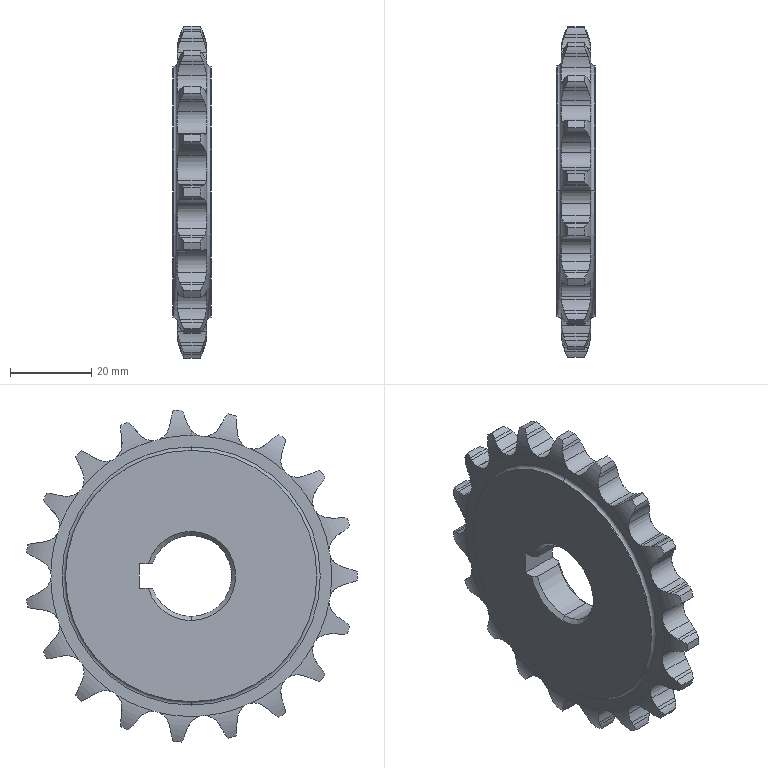Part | SolidWorks | features Chamfer 3, Cut 2, Revolution 2, CirPattern 1 | 1 solid | 225 faces | box 9.37 x 81.595 x 81.862 mm | volume 34307 mm3 | cylinder 130 | plane 45 | torus 44 | cone 6 | commonest cylinder face diameters 11.518 x40 20.732 x40 8.06 x24 82 x19 62 x4 20 x3